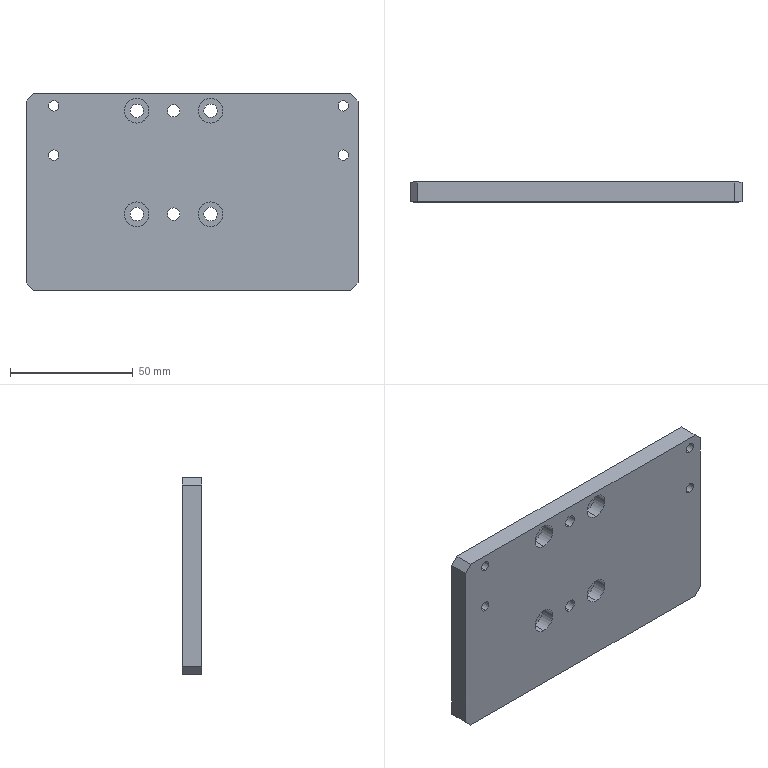Part | SolidWorks | features HoleWzd 3, Chamfer 1, Extrusion 1 | 1 solid | 42 faces | box 135 x 8 x 80 mm | volume 83489 mm3 | cylinder 28 | plane 14 | commonest cylinder face diameters 4.2 x8 5.5 x8 10 x8 5 x4
STEP:
#1=CARTESIAN_POINT('',(60.05,8.,-4.5));
#2=VERTEX_POINT('',#1);
#3=CARTESIAN_POINT('',(60.05,8.,-9.5));
#4=VERTEX_POINT('',#3);
#5=CARTESIAN_POINT('',(60.05,8.,-7.));
#6=DIRECTION('',(0.,-1.,0.));
#7=DIRECTION('',(0.,0.,-1.));
#8=AXIS2_PLACEMENT_3D('',#5,#6,#7);
#9=CIRCLE('',#8,2.5);
#10=EDGE_CURVE('',#2,#4,#9,.T.);
#11=ORIENTED_EDGE('',*,*,#10,.F.);
#12=CARTESIAN_POINT('',(60.05,0.,-4.5));
#13=VERTEX_POINT('',#12);
#14=CARTESIAN_POINT('',(60.05,0.,-4.5));
#15=DIRECTION('',(0.,-1.,0.));
#16=VECTOR('',#15,1000.);
#17=LINE('',#14,#16);
#18=EDGE_CURVE('',#2,#13,#17,.T.);
#19=ORIENTED_EDGE('',*,*,#18,.T.);
#20=CARTESIAN_POINT('',(60.05,0.,-9.5));
#21=VERTEX_POINT('',#20);
#22=CARTESIAN_POINT('',(60.05,0.,-7.));
#23=DIRECTION('',(0.,-1.,0.));
#24=DIRECTION('',(0.,0.,-1.));
#25=AXIS2_PLACEMENT_3D('',#22,#23,#24);
#26=CIRCLE('',#25,2.5);
#27=EDGE_CURVE('',#13,#21,#26,.T.);
#28=ORIENTED_EDGE('',*,*,#27,.T.);
#29=CARTESIAN_POINT('',(60.05,0.,-9.5));
#30=DIRECTION('',(0.,-1.,0.));
#31=VECTOR('',#30,1000.);
#32=LINE('',#29,#31);
#33=EDGE_CURVE('',#4,#21,#32,.T.);
#34=ORIENTED_EDGE('',*,*,#33,.F.);
#35=EDGE_LOOP('',(#11,#19,#28,#34));
#36=FACE_OUTER_BOUND('',#35,.T.);
#37=CARTESIAN_POINT('',(60.05,0.,-7.));
#38=DIRECTION('',(0.,-1.,0.));
#39=DIRECTION('',(0.,0.,-1.));
#40=AXIS2_PLACEMENT_3D('',#37,#38,#39);
#41=CYLINDRICAL_SURFACE('',#40,2.5);
#42=ADVANCED_FACE('',(#36),#41,.F.);
#43=CARTESIAN_POINT('',(60.05,8.,-46.5));
#44=VERTEX_POINT('',#43);
#45=CARTESIAN_POINT('',(60.05,8.,-51.5));
#46=VERTEX_POINT('',#45);
#47=CARTESIAN_POINT('',(60.05,8.,-49.));
#48=DIRECTION('',(0.,-1.,0.));
#49=DIRECTION('',(0.,0.,-1.));
#50=AXIS2_PLACEMENT_3D('',#47,#48,#49);
#51=CIRCLE('',#50,2.5);
#52=EDGE_CURVE('',#44,#46,#51,.T.);
#53=ORIENTED_EDGE('',*,*,#52,.F.);
#54=CARTESIAN_POINT('',(60.05,0.,-46.5));
#55=VERTEX_POINT('',#54);
#56=CARTESIAN_POINT('',(60.05,0.,-46.5));
#57=DIRECTION('',(0.,-1.,0.));
#58=VECTOR('',#57,1000.);
#59=LINE('',#56,#58);
#60=EDGE_CURVE('',#44,#55,#59,.T.);
#61=ORIENTED_EDGE('',*,*,#60,.T.);
#62=CARTESIAN_POINT('',(60.05,0.,-51.5));
#63=VERTEX_POINT('',#62);
#64=CARTESIAN_POINT('',(60.05,0.,-49.));
#65=DIRECTION('',(0.,-1.,0.));
#66=DIRECTION('',(0.,0.,-1.));
#67=AXIS2_PLACEMENT_3D('',#64,#65,#66);
#68=CIRCLE('',#67,2.5);
#69=EDGE_CURVE('',#55,#63,#68,.T.);
#70=ORIENTED_EDGE('',*,*,#69,.T.);
#71=CARTESIAN_POINT('',(60.05,0.,-51.5));
#72=DIRECTION('',(0.,-1.,0.));
#73=VECTOR('',#72,1000.);
#74=LINE('',#71,#73);
#75=EDGE_CURVE('',#46,#63,#74,.T.);
#76=ORIENTED_EDGE('',*,*,#75,.F.);
#77=EDGE_LOOP('',(#53,#61,#70,#76));
#78=FACE_OUTER_BOUND('',#77,.T.);
#79=CARTESIAN_POINT('',(60.05,0.,-49.));
#80=DIRECTION('',(0.,-1.,0.));
#81=DIRECTION('',(0.,0.,-1.));
#82=AXIS2_PLACEMENT_3D('',#79,#80,#81);
#83=CYLINDRICAL_SURFACE('',#82,2.5);
#84=ADVANCED_FACE('',(#78),#83,.F.);
#85=CARTESIAN_POINT('',(129.,0.,-27.1));
#86=VERTEX_POINT('',#85);
#87=CARTESIAN_POINT('',(129.,0.,-22.9));
#88=VERTEX_POINT('',#87);
#89=CARTESIAN_POINT('',(129.,0.,-25.));
#90=DIRECTION('',(0.,1.,0.));
#91=DIRECTION('',(0.,0.,1.));
#92=AXIS2_PLACEMENT_3D('',#89,#90,#91);
#93=CIRCLE('',#92,2.1);
#94=EDGE_CURVE('',#86,#88,#93,.T.);
#95=ORIENTED_EDGE('',*,*,#94,.F.);
#96=CARTESIAN_POINT('',(129.,8.,-27.1));
#97=VERTEX_POINT('',#96);
#98=CARTESIAN_POINT('',(129.,8.,-27.1));
#99=DIRECTION('',(0.,1.,0.));
#100=VECTOR('',#99,1000.);
#101=LINE('',#98,#100);
#102=EDGE_CURVE('',#86,#97,#101,.T.);
#103=ORIENTED_EDGE('',*,*,#102,.T.);
#104=CARTESIAN_POINT('',(129.,8.,-22.9));
#105=VERTEX_POINT('',#104);
#106=CARTESIAN_POINT('',(129.,8.,-25.));
#107=DIRECTION('',(0.,1.,0.));
#108=DIRECTION('',(0.,0.,1.));
#109=AXIS2_PLACEMENT_3D('',#106,#107,#108);
#110=CIRCLE('',#109,2.1);
#111=EDGE_CURVE('',#97,#105,#110,.T.);
#112=ORIENTED_EDGE('',*,*,#111,.T.);
#113=CARTESIAN_POINT('',(129.,8.,-22.9));
#114=DIRECTION('',(0.,1.,0.));
#115=VECTOR('',#114,1000.);
#116=LINE('',#113,#115);
#117=EDGE_CURVE('',#88,#105,#116,.T.);
#118=ORIENTED_EDGE('',*,*,#117,.F.);
#119=EDGE_LOOP('',(#95,#103,#112,#118));
#120=FACE_OUTER_BOUND('',#119,.T.);
#121=CARTESIAN_POINT('',(129.,8.,-25.));
#122=DIRECTION('',(0.,1.,0.));
#123=DIRECTION('',(0.,0.,1.));
#124=AXIS2_PLACEMENT_3D('',#121,#122,#123);
#125=CYLINDRICAL_SURFACE('',#124,2.1);
#126=ADVANCED_FACE('',(#120),#125,.F.);
#127=CARTESIAN_POINT('',(129.,0.,-7.1));
#128=VERTEX_POINT('',#127);
#129=CARTESIAN_POINT('',(129.,0.,-2.9));
#130=VERTEX_POINT('',#129);
#131=CARTESIAN_POINT('',(129.,0.,-5.));
#132=DIRECTION('',(0.,1.,0.));
#133=DIRECTION('',(0.,0.,1.));
#134=AXIS2_PLACEMENT_3D('',#131,#132,#133);
#135=CIRCLE('',#134,2.1);
#136=EDGE_CURVE('',#128,#130,#135,.T.);
#137=ORIENTED_EDGE('',*,*,#136,.F.);
#138=CARTESIAN_POINT('',(129.,8.,-7.1));
#139=VERTEX_POINT('',#138);
#140=CARTESIAN_POINT('',(129.,8.,-7.1));
#141=DIRECTION('',(0.,1.,0.));
#142=VECTOR('',#141,1000.);
#143=LINE('',#140,#142);
#144=EDGE_CURVE('',#128,#139,#143,.T.);
#145=ORIENTED_EDGE('',*,*,#144,.T.);
#146=CARTESIAN_POINT('',(129.,8.,-2.9));
#147=VERTEX_POINT('',#146);
#148=CARTESIAN_POINT('',(129.,8.,-5.));
#149=DIRECTION('',(0.,1.,0.));
#150=DIRECTION('',(0.,0.,1.));
#151=AXIS2_PLACEMENT_3D('',#148,#149,#150);
#152=CIRCLE('',#151,2.1);
#153=EDGE_CURVE('',#139,#147,#152,.T.);
#154=ORIENTED_EDGE('',*,*,#153,.T.);
#155=CARTESIAN_POINT('',(129.,8.,-2.9));
#156=DIRECTION('',(0.,1.,0.));
#157=VECTOR('',#156,1000.);
#158=LINE('',#155,#157);
#159=EDGE_CURVE('',#130,#147,#158,.T.);
#160=ORIENTED_EDGE('',*,*,#159,.F.);
#161=EDGE_LOOP('',(#137,#145,#154,#160));
#162=FACE_OUTER_BOUND('',#161,.T.);
#163=CARTESIAN_POINT('',(129.,8.,-5.));
#164=DIRECTION('',(0.,1.,0.));
#165=DIRECTION('',(0.,0.,1.));
#166=AXIS2_PLACEMENT_3D('',#163,#164,#165);
#167=CYLINDRICAL_SURFACE('',#166,2.1);
#168=ADVANCED_FACE('',(#162),#167,.F.);
#169=CARTESIAN_POINT('',(11.3,0.,-27.1));
#170=VERTEX_POINT('',#169);
#171=CARTESIAN_POINT('',(11.3,0.,-22.9));
#172=VERTEX_POINT('',#171);
#173=CARTESIAN_POINT('',(11.3,0.,-25.));
#174=DIRECTION('',(0.,1.,0.));
#175=DIRECTION('',(0.,0.,1.));
#176=AXIS2_PLACEMENT_3D('',#173,#174,#175);
#177=CIRCLE('',#176,2.1);
#178=EDGE_CURVE('',#170,#172,#177,.T.);
#179=ORIENTED_EDGE('',*,*,#178,.F.);
#180=CARTESIAN_POINT('',(11.3,8.,-27.1));
#181=VERTEX_POINT('',#180);
#182=CARTESIAN_POINT('',(11.3,8.,-27.1));
#183=DIRECTION('',(0.,1.,0.));
#184=VECTOR('',#183,1000.);
#185=LINE('',#182,#184);
#186=EDGE_CURVE('',#170,#181,#185,.T.);
#187=ORIENTED_EDGE('',*,*,#186,.T.);
#188=CARTESIAN_POINT('',(11.3,8.,-22.9));
#189=VERTEX_POINT('',#188);
#190=CARTESIAN_POINT('',(11.3,8.,-25.));
#191=DIRECTION('',(0.,1.,0.));
#192=DIRECTION('',(0.,0.,1.));
#193=AXIS2_PLACEMENT_3D('',#190,#191,#192);
#194=CIRCLE('',#193,2.1);
#195=EDGE_CURVE('',#181,#189,#194,.T.);
#196=ORIENTED_EDGE('',*,*,#195,.T.);
#197=CARTESIAN_POINT('',(11.3,8.,-22.9));
#198=DIRECTION('',(0.,1.,0.));
#199=VECTOR('',#198,1000.);
#200=LINE('',#197,#199);
#201=EDGE_CURVE('',#172,#189,#200,.T.);
#202=ORIENTED_EDGE('',*,*,#201,.F.);
#203=EDGE_LOOP('',(#179,#187,#196,#202));
#204=FACE_OUTER_BOUND('',#203,.T.);
#205=CARTESIAN_POINT('',(11.3,8.,-25.));
#206=DIRECTION('',(0.,1.,0.));
#207=DIRECTION('',(0.,0.,1.));
#208=AXIS2_PLACEMENT_3D('',#205,#206,#207);
#209=CYLINDRICAL_SURFACE('',#208,2.1);
#210=ADVANCED_FACE('',(#204),#209,.F.);
#211=CARTESIAN_POINT('',(11.3,0.,-7.1));
#212=VERTEX_POINT('',#211);
#213=CARTESIAN_POINT('',(11.3,0.,-2.9));
#214=VERTEX_POINT('',#213);
#215=CARTESIAN_POINT('',(11.3,0.,-5.));
#216=DIRECTION('',(0.,1.,0.));
#217=DIRECTION('',(0.,0.,1.));
#218=AXIS2_PLACEMENT_3D('',#215,#216,#217);
#219=CIRCLE('',#218,2.1);
#220=EDGE_CURVE('',#212,#214,#219,.T.);
#221=ORIENTED_EDGE('',*,*,#220,.F.);
#222=CARTESIAN_POINT('',(11.3,8.,-7.1));
#223=VERTEX_POINT('',#222);
#224=CARTESIAN_POINT('',(11.3,8.,-7.1));
#225=DIRECTION('',(0.,1.,0.));
#226=VECTOR('',#225,1000.);
#227=LINE('',#224,#226);
#228=EDGE_CURVE('',#212,#223,#227,.T.);
#229=ORIENTED_EDGE('',*,*,#228,.T.);
#230=CARTESIAN_POINT('',(11.3,8.,-2.9));
#231=VERTEX_POINT('',#230);
#232=CARTESIAN_POINT('',(11.3,8.,-5.));
#233=DIRECTION('',(0.,1.,0.));
#234=DIRECTION('',(0.,0.,1.));
#235=AXIS2_PLACEMENT_3D('',#232,#233,#234);
#236=CIRCLE('',#235,2.1);
#237=EDGE_CURVE('',#223,#231,#236,.T.);
#238=ORIENTED_EDGE('',*,*,#237,.T.);
#239=CARTESIAN_POINT('',(11.3,8.,-2.9));
#240=DIRECTION('',(0.,1.,0.));
#241=VECTOR('',#240,1000.);
#242=LINE('',#239,#241);
#243=EDGE_CURVE('',#214,#231,#242,.T.);
#244=ORIENTED_EDGE('',*,*,#243,.F.);
#245=EDGE_LOOP('',(#221,#229,#238,#244));
#246=FACE_OUTER_BOUND('',#245,.T.);
#247=CARTESIAN_POINT('',(11.3,8.,-5.));
#248=DIRECTION('',(0.,1.,0.));
#249=DIRECTION('',(0.,0.,1.));
#250=AXIS2_PLACEMENT_3D('',#247,#248,#249);
#251=CYLINDRICAL_SURFACE('',#250,2.1);
#252=ADVANCED_FACE('',(#246),#251,.F.);
#253=CARTESIAN_POINT('',(75.05,5.7,-44.));
#254=VERTEX_POINT('',#253);
#255=CARTESIAN_POINT('',(75.05,5.7,-54.));
#256=VERTEX_POINT('',#255);
#257=CARTESIAN_POINT('',(75.05,5.7,-49.));
#258=DIRECTION('',(0.,-1.,0.));
#259=DIRECTION('',(0.,0.,-1.));
#260=AXIS2_PLACEMENT_3D('',#257,#258,#259);
#261=CIRCLE('',#260,5.);
#262=EDGE_CURVE('',#254,#256,#261,.T.);
#263=ORIENTED_EDGE('',*,*,#262,.F.);
#264=CARTESIAN_POINT('',(75.05,0.,-44.));
#265=VERTEX_POINT('',#264);
#266=CARTESIAN_POINT('',(75.05,0.,-44.));
#267=DIRECTION('',(0.,-1.,0.));
#268=VECTOR('',#267,1000.);
#269=LINE('',#266,#268);
#270=EDGE_CURVE('',#254,#265,#269,.T.);
#271=ORIENTED_EDGE('',*,*,#270,.T.);
#272=CARTESIAN_POINT('',(75.05,0.,-54.));
#273=VERTEX_POINT('',#272);
#274=CARTESIAN_POINT('',(75.05,0.,-49.));
#275=DIRECTION('',(0.,-1.,0.));
#276=DIRECTION('',(0.,0.,-1.));
#277=AXIS2_PLACEMENT_3D('',#274,#275,#276);
#278=CIRCLE('',#277,5.);
#279=EDGE_CURVE('',#265,#273,#278,.T.);
#280=ORIENTED_EDGE('',*,*,#279,.T.);
#281=CARTESIAN_POINT('',(75.05,0.,-54.));
#282=DIRECTION('',(0.,-1.,0.));
#283=VECTOR('',#282,1000.);
#284=LINE('',#281,#283);
#285=EDGE_CURVE('',#256,#273,#284,.T.);
#286=ORIENTED_EDGE('',*,*,#285,.F.);
#287=EDGE_LOOP('',(#263,#271,#280,#286));
#288=FACE_OUTER_BOUND('',#287,.T.);
#289=CARTESIAN_POINT('',(75.05,0.,-49.));
#290=DIRECTION('',(0.,-1.,0.));
#291=DIRECTION('',(0.,0.,-1.));
#292=AXIS2_PLACEMENT_3D('',#289,#290,#291);
#293=CYLINDRICAL_SURFACE('',#292,5.);
#294=ADVANCED_FACE('',(#288),#293,.F.);
#295=CARTESIAN_POINT('',(75.05,8.,-46.25));
#296=VERTEX_POINT('',#295);
#297=CARTESIAN_POINT('',(75.05,8.,-51.75));
#298=VERTEX_POINT('',#297);
#299=CARTESIAN_POINT('',(75.05,8.,-49.));
#300=DIRECTION('',(0.,-1.,0.));
#301=DIRECTION('',(0.,0.,-1.));
#302=AXIS2_PLACEMENT_3D('',#299,#300,#301);
#303=CIRCLE('',#302,2.75);
#304=EDGE_CURVE('',#296,#298,#303,.T.);
#305=ORIENTED_EDGE('',*,*,#304,.F.);
#306=CARTESIAN_POINT('',(75.05,5.7,-46.25));
#307=VERTEX_POINT('',#306);
#308=CARTESIAN_POINT('',(75.05,0.,-46.25));
#309=DIRECTION('',(0.,-1.,0.));
#310=VECTOR('',#309,1000.);
#311=LINE('',#308,#310);
#312=EDGE_CURVE('',#296,#307,#311,.T.);
#313=ORIENTED_EDGE('',*,*,#312,.T.);
#314=CARTESIAN_POINT('',(75.05,5.7,-51.75));
#315=VERTEX_POINT('',#314);
#316=CARTESIAN_POINT('',(75.05,5.7,-49.));
#317=DIRECTION('',(0.,-1.,0.));
#318=DIRECTION('',(0.,0.,-1.));
#319=AXIS2_PLACEMENT_3D('',#316,#317,#318);
#320=CIRCLE('',#319,2.75);
#321=EDGE_CURVE('',#307,#315,#320,.T.);
#322=ORIENTED_EDGE('',*,*,#321,.T.);
#323=CARTESIAN_POINT('',(75.05,0.,-51.75));
#324=DIRECTION('',(0.,-1.,0.));
#325=VECTOR('',#324,1000.);
#326=LINE('',#323,#325);
#327=EDGE_CURVE('',#298,#315,#326,.T.);
#328=ORIENTED_EDGE('',*,*,#327,.F.);
#329=EDGE_LOOP('',(#305,#313,#322,#328));
#330=FACE_OUTER_BOUND('',#329,.T.);
#331=CARTESIAN_POINT('',(75.05,0.,-49.));
#332=DIRECTION('',(0.,-1.,0.));
#333=DIRECTION('',(0.,0.,-1.));
#334=AXIS2_PLACEMENT_3D('',#331,#332,#333);
#335=CYLINDRICAL_SURFACE('',#334,2.75);
#336=ADVANCED_FACE('',(#330),#335,.F.);
#337=CARTESIAN_POINT('',(45.05,5.7,-44.));
#338=VERTEX_POINT('',#337);
#339=CARTESIAN_POINT('',(45.05,5.7,-54.));
#340=VERTEX_POINT('',#339);
#341=CARTESIAN_POINT('',(45.05,5.7,-49.));
#342=DIRECTION('',(0.,-1.,0.));
#343=DIRECTION('',(0.,0.,-1.));
#344=AXIS2_PLACEMENT_3D('',#341,#342,#343);
#345=CIRCLE('',#344,5.);
#346=EDGE_CURVE('',#338,#340,#345,.T.);
#347=ORIENTED_EDGE('',*,*,#346,.F.);
#348=CARTESIAN_POINT('',(45.05,0.,-44.));
#349=VERTEX_POINT('',#348);
#350=CARTESIAN_POINT('',(45.05,0.,-44.));
#351=DIRECTION('',(0.,-1.,0.));
#352=VECTOR('',#351,1000.);
#353=LINE('',#350,#352);
#354=EDGE_CURVE('',#338,#349,#353,.T.);
#355=ORIENTED_EDGE('',*,*,#354,.T.);
#356=CARTESIAN_POINT('',(45.05,0.,-54.));
#357=VERTEX_POINT('',#356);
#358=CARTESIAN_POINT('',(45.05,0.,-49.));
#359=DIRECTION('',(0.,-1.,0.));
#360=DIRECTION('',(0.,0.,-1.));
#361=AXIS2_PLACEMENT_3D('',#358,#359,#360);
#362=CIRCLE('',#361,5.);
#363=EDGE_CURVE('',#349,#357,#362,.T.);
#364=ORIENTED_EDGE('',*,*,#363,.T.);
#365=CARTESIAN_POINT('',(45.05,0.,-54.));
#366=DIRECTION('',(0.,-1.,0.));
#367=VECTOR('',#366,1000.);
#368=LINE('',#365,#367);
#369=EDGE_CURVE('',#340,#357,#368,.T.);
#370=ORIENTED_EDGE('',*,*,#369,.F.);
#371=EDGE_LOOP('',(#347,#355,#364,#370));
#372=FACE_OUTER_BOUND('',#371,.T.);
#373=CARTESIAN_POINT('',(45.05,0.,-49.));
#374=DIRECTION('',(0.,-1.,0.));
#375=DIRECTION('',(0.,0.,-1.));
#376=AXIS2_PLACEMENT_3D('',#373,#374,#375);
#377=CYLINDRICAL_SURFACE('',#376,5.);
#378=ADVANCED_FACE('',(#372),#377,.F.);
#379=CARTESIAN_POINT('',(45.05,8.,-46.25));
#380=VERTEX_POINT('',#379);
#381=CARTESIAN_POINT('',(45.05,8.,-51.75));
#382=VERTEX_POINT('',#381);
#383=CARTESIAN_POINT('',(45.05,8.,-49.));
#384=DIRECTION('',(0.,-1.,0.));
#385=DIRECTION('',(0.,0.,-1.));
#386=AXIS2_PLACEMENT_3D('',#383,#384,#385);
#387=CIRCLE('',#386,2.75);
#388=EDGE_CURVE('',#380,#382,#387,.T.);
#389=ORIENTED_EDGE('',*,*,#388,.F.);
#390=CARTESIAN_POINT('',(45.05,5.7,-46.25));
#391=VERTEX_POINT('',#390);
#392=CARTESIAN_POINT('',(45.05,0.,-46.25));
#393=DIRECTION('',(0.,-1.,0.));
#394=VECTOR('',#393,1000.);
#395=LINE('',#392,#394);
#396=EDGE_CURVE('',#380,#391,#395,.T.);
#397=ORIENTED_EDGE('',*,*,#396,.T.);
#398=CARTESIAN_POINT('',(45.05,5.7,-51.75));
#399=VERTEX_POINT('',#398);
#400=CARTESIAN_POINT('',(45.05,5.7,-49.));
#401=DIRECTION('',(0.,-1.,0.));
#402=DIRECTION('',(0.,0.,-1.));
#403=AXIS2_PLACEMENT_3D('',#400,#401,#402);
#404=CIRCLE('',#403,2.75);
#405=EDGE_CURVE('',#391,#399,#404,.T.);
#406=ORIENTED_EDGE('',*,*,#405,.T.);
#407=CARTESIAN_POINT('',(45.05,0.,-51.75));
#408=DIRECTION('',(0.,-1.,0.));
#409=VECTOR('',#408,1000.);
#410=LINE('',#407,#409);
#411=EDGE_CURVE('',#382,#399,#410,.T.);
#412=ORIENTED_EDGE('',*,*,#411,.F.);
#413=EDGE_LOOP('',(#389,#397,#406,#412));
#414=FACE_OUTER_BOUND('',#413,.T.);
#415=CARTESIAN_POINT('',(45.05,0.,-49.));
#416=DIRECTION('',(0.,-1.,0.));
#417=DIRECTION('',(0.,0.,-1.));
#418=AXIS2_PLACEMENT_3D('',#415,#416,#417);
#419=CYLINDRICAL_SURFACE('',#418,2.75);
#420=ADVANCED_FACE('',(#414),#419,.F.);
#421=CARTESIAN_POINT('',(45.05,5.7,-2.));
#422=VERTEX_POINT('',#421);
#423=CARTESIAN_POINT('',(45.05,5.7,-12.));
#424=VERTEX_POINT('',#423);
#425=CARTESIAN_POINT('',(45.05,5.7,-7.));
#426=DIRECTION('',(0.,-1.,0.));
#427=DIRECTION('',(0.,0.,-1.));
#428=AXIS2_PLACEMENT_3D('',#425,#426,#427);
#429=CIRCLE('',#428,5.);
#430=EDGE_CURVE('',#422,#424,#429,.T.);
#431=ORIENTED_EDGE('',*,*,#430,.F.);
#432=CARTESIAN_POINT('',(45.05,0.,-2.));
#433=VERTEX_POINT('',#432);
#434=CARTESIAN_POINT('',(45.05,0.,-2.));
#435=DIRECTION('',(0.,-1.,0.));
#436=VECTOR('',#435,1000.);
#437=LINE('',#434,#436);
#438=EDGE_CURVE('',#422,#433,#437,.T.);
#439=ORIENTED_EDGE('',*,*,#438,.T.);
#440=CARTESIAN_POINT('',(45.05,0.,-12.));
#441=VERTEX_POINT('',#440);
#442=CARTESIAN_POINT('',(45.05,0.,-7.));
#443=DIRECTION('',(0.,-1.,0.));
#444=DIRECTION('',(0.,0.,-1.));
#445=AXIS2_PLACEMENT_3D('',#442,#443,#444);
#446=CIRCLE('',#445,5.);
#447=EDGE_CURVE('',#433,#441,#446,.T.);
#448=ORIENTED_EDGE('',*,*,#447,.T.);
#449=CARTESIAN_POINT('',(45.05,0.,-12.));
#450=DIRECTION('',(0.,-1.,0.));
#451=VECTOR('',#450,1000.);
#452=LINE('',#449,#451);
#453=EDGE_CURVE('',#424,#441,#452,.T.);
#454=ORIENTED_EDGE('',*,*,#453,.F.);
#455=EDGE_LOOP('',(#431,#439,#448,#454));
#456=FACE_OUTER_BOUND('',#455,.T.);
#457=CARTESIAN_POINT('',(45.05,0.,-7.));
#458=DIRECTION('',(0.,-1.,0.));
#459=DIRECTION('',(0.,0.,-1.));
#460=AXIS2_PLACEMENT_3D('',#457,#458,#459);
#461=CYLINDRICAL_SURFACE('',#460,5.);
#462=ADVANCED_FACE('',(#456),#461,.F.);
#463=CARTESIAN_POINT('',(45.05,8.,-4.25));
#464=VERTEX_POINT('',#463);
#465=CARTESIAN_POINT('',(45.05,8.,-9.75));
#466=VERTEX_POINT('',#465);
#467=CARTESIAN_POINT('',(45.05,8.,-7.));
#468=DIRECTION('',(0.,-1.,0.));
#469=DIRECTION('',(0.,0.,-1.));
#470=AXIS2_PLACEMENT_3D('',#467,#468,#469);
#471=CIRCLE('',#470,2.75);
#472=EDGE_CURVE('',#464,#466,#471,.T.);
#473=ORIENTED_EDGE('',*,*,#472,.F.);
#474=CARTESIAN_POINT('',(45.05,5.7,-4.25));
#475=VERTEX_POINT('',#474);
#476=CARTESIAN_POINT('',(45.05,0.,-4.25));
#477=DIRECTION('',(0.,-1.,0.));
#478=VECTOR('',#477,1000.);
#479=LINE('',#476,#478);
#480=EDGE_CURVE('',#464,#475,#479,.T.);
#481=ORIENTED_EDGE('',*,*,#480,.T.);
#482=CARTESIAN_POINT('',(45.05,5.7,-9.75));
#483=VERTEX_POINT('',#482);
#484=CARTESIAN_POINT('',(45.05,5.7,-7.));
#485=DIRECTION('',(0.,-1.,0.));
#486=DIRECTION('',(0.,0.,-1.));
#487=AXIS2_PLACEMENT_3D('',#484,#485,#486);
#488=CIRCLE('',#487,2.75);
#489=EDGE_CURVE('',#475,#483,#488,.T.);
#490=ORIENTED_EDGE('',*,*,#489,.T.);
#491=CARTESIAN_POINT('',(45.05,0.,-9.75));
#492=DIRECTION('',(0.,-1.,0.));
#493=VECTOR('',#492,1000.);
#494=LINE('',#491,#493);
#495=EDGE_CURVE('',#466,#483,#494,.T.);
#496=ORIENTED_EDGE('',*,*,#495,.F.);
#497=EDGE_LOOP('',(#473,#481,#490,#496));
#498=FACE_OUTER_BOUND('',#497,.T.);
#499=CARTESIAN_POINT('',(45.05,0.,-7.));
#500=DIRECTION('',(0.,-1.,0.));
#501=DIRECTION('',(0.,0.,-1.));
#502=AXIS2_PLACEMENT_3D('',#499,#500,#501);
#503=CYLINDRICAL_SURFACE('',#502,2.75);
#504=ADVANCED_FACE('',(#498),#503,.F.);
#505=CARTESIAN_POINT('',(75.05,5.7,-2.));
#506=VERTEX_POINT('',#505);
#507=CARTESIAN_POINT('',(75.05,5.7,-12.));
#508=VERTEX_POINT('',#507);
#509=CARTESIAN_POINT('',(75.05,5.7,-7.));
#510=DIRECTION('',(0.,-1.,0.));
#511=DIRECTION('',(0.,0.,-1.));
#512=AXIS2_PLACEMENT_3D('',#509,#510,#511);
#513=CIRCLE('',#512,5.);
#514=EDGE_CURVE('',#506,#508,#513,.T.);
#515=ORIENTED_EDGE('',*,*,#514,.F.);
#516=CARTESIAN_POINT('',(75.05,0.,-2.));
#517=VERTEX_POINT('',#516);
#518=CARTESIAN_POINT('',(75.05,0.,-2.));
#519=DIRECTION('',(0.,-1.,0.));
#520=VECTOR('',#519,1000.);
#521=LINE('',#518,#520);
#522=EDGE_CURVE('',#506,#517,#521,.T.);
#523=ORIENTED_EDGE('',*,*,#522,.T.);
#524=CARTESIAN_POINT('',(75.05,0.,-12.));
#525=VERTEX_POINT('',#524);
#526=CARTESIAN_POINT('',(75.05,0.,-7.));
#527=DIRECTION('',(0.,-1.,0.));
#528=DIRECTION('',(0.,0.,-1.));
#529=AXIS2_PLACEMENT_3D('',#526,#527,#528);
#530=CIRCLE('',#529,5.);
#531=EDGE_CURVE('',#517,#525,#530,.T.);
#532=ORIENTED_EDGE('',*,*,#531,.T.);
#533=CARTESIAN_POINT('',(75.05,0.,-12.));
#534=DIRECTION('',(0.,-1.,0.));
#535=VECTOR('',#534,1000.);
#536=LINE('',#533,#535);
#537=EDGE_CURVE('',#508,#525,#536,.T.);
#538=ORIENTED_EDGE('',*,*,#537,.F.);
#539=EDGE_LOOP('',(#515,#523,#532,#538));
#540=FACE_OUTER_BOUND('',#539,.T.);
#541=CARTESIAN_POINT('',(75.05,0.,-7.));
#542=DIRECTION('',(0.,-1.,0.));
#543=DIRECTION('',(0.,0.,-1.));
#544=AXIS2_PLACEMENT_3D('',#541,#542,#543);
#545=CYLINDRICAL_SURFACE('',#544,5.);
#546=ADVANCED_FACE('',(#540),#545,.F.);
#547=CARTESIAN_POINT('',(75.05,8.,-4.25));
#548=VERTEX_POINT('',#547);
#549=CARTESIAN_POINT('',(75.05,8.,-9.75));
#550=VERTEX_POINT('',#549);
#551=CARTESIAN_POINT('',(75.05,8.,-7.));
#552=DIRECTION('',(0.,-1.,0.));
#553=DIRECTION('',(0.,0.,-1.));
#554=AXIS2_PLACEMENT_3D('',#551,#552,#553);
#555=CIRCLE('',#554,2.75);
#556=EDGE_CURVE('',#548,#550,#555,.T.);
#557=ORIENTED_EDGE('',*,*,#556,.F.);
#558=CARTESIAN_POINT('',(75.05,5.7,-4.25));
#559=VERTEX_POINT('',#558);
#560=CARTESIAN_POINT('',(75.05,0.,-4.25));
#561=DIRECTION('',(0.,-1.,0.));
#562=VECTOR('',#561,1000.);
#563=LINE('',#560,#562);
#564=EDGE_CURVE('',#548,#559,#563,.T.);
#565=ORIENTED_EDGE('',*,*,#564,.T.);
#566=CARTESIAN_POINT('',(75.05,5.7,-9.75));
#567=VERTEX_POINT('',#566);
#568=CARTESIAN_POINT('',(75.05,5.7,-7.));
#569=DIRECTION('',(0.,-1.,0.));
#570=DIRECTION('',(0.,0.,-1.));
#571=AXIS2_PLACEMENT_3D('',#568,#569,#570);
#572=CIRCLE('',#571,2.75);
#573=EDGE_CURVE('',#559,#567,#572,.T.);
#574=ORIENTED_EDGE('',*,*,#573,.T.);
#575=CARTESIAN_POINT('',(75.05,0.,-9.75));
#576=DIRECTION('',(0.,-1.,0.));
#577=VECTOR('',#576,1000.);
#578=LINE('',#575,#577);
#579=EDGE_CURVE('',#550,#567,#578,.T.);
#580=ORIENTED_EDGE('',*,*,#579,.F.);
#581=EDGE_LOOP('',(#557,#565,#574,#580));
#582=FACE_OUTER_BOUND('',#581,.T.);
#583=CARTESIAN_POINT('',(75.05,0.,-7.));
#584=DIRECTION('',(0.,-1.,0.));
#585=DIRECTION('',(0.,0.,-1.));
#586=AXIS2_PLACEMENT_3D('',#583,#584,#585);
#587=CYLINDRICAL_SURFACE('',#586,2.75);
#588=ADVANCED_FACE('',(#582),#587,.F.);
#589=CARTESIAN_POINT('',(0.,0.,-77.));
#590=VERTEX_POINT('',#589);
#591=CARTESIAN_POINT('',(0.,0.,-3.));
#592=VERTEX_POINT('',#591);
#593=CARTESIAN_POINT('',(0.,0.,0.));
#594=DIRECTION('',(0.,0.,1.));
#595=VECTOR('',#594,1000.);
#596=LINE('',#593,#595);
#597=EDGE_CURVE('',#590,#592,#596,.T.);
#598=ORIENTED_EDGE('',*,*,#597,.T.);
#599=CARTESIAN_POINT('',(0.,8.,-3.));
#600=VERTEX_POINT('',#599);
#601=CARTESIAN_POINT('',(0.,8.,-3.));
#602=DIRECTION('',(0.,1.,0.));
#603=VECTOR('',#602,1000.);
#604=LINE('',#601,#603);
#605=EDGE_CURVE('',#592,#600,#604,.T.);
#606=ORIENTED_EDGE('',*,*,#605,.T.);
#607=CARTESIAN_POINT('',(0.,8.,-77.));
#608=VERTEX_POINT('',#607);
#609=CARTESIAN_POINT('',(0.,8.,0.));
#610=DIRECTION('',(0.,0.,1.));
#611=VECTOR('',#610,1000.);
#612=LINE('',#609,#611);
#613=EDGE_CURVE('',#608,#600,#612,.T.);
#614=ORIENTED_EDGE('',*,*,#613,.F.);
#615=CARTESIAN_POINT('',(0.,8.,-77.));
#616=DIRECTION('',(0.,-1.,0.));
#617=VECTOR('',#616,1000.);
#618=LINE('',#615,#617);
#619=EDGE_CURVE('',#608,#590,#618,.T.);
#620=ORIENTED_EDGE('',*,*,#619,.T.);
#621=EDGE_LOOP('',(#598,#606,#614,#620));
#622=FACE_OUTER_BOUND('',#621,.T.);
#623=CARTESIAN_POINT('',(0.,8.,0.));
#624=DIRECTION('',(1.,0.,0.));
#625=DIRECTION('',(0.,0.,-1.));
#626=AXIS2_PLACEMENT_3D('',#623,#624,#625);
#627=PLANE('',#626);
#628=ADVANCED_FACE('',(#622),#627,.F.);
#629=CARTESIAN_POINT('',(3.,8.,0.));
#630=VERTEX_POINT('',#629);
#631=CARTESIAN_POINT('',(132.,8.,0.));
#632=VERTEX_POINT('',#631);
#633=CARTESIAN_POINT('',(0.,8.,0.));
#634=DIRECTION('',(1.,0.,0.));
#635=VECTOR('',#634,1000.);
#636=LINE('',#633,#635);
#637=EDGE_CURVE('',#630,#632,#636,.T.);
#638=ORIENTED_EDGE('',*,*,#637,.F.);
#639=CARTESIAN_POINT('',(3.,0.,0.));
#640=VERTEX_POINT('',#639);
#641=CARTESIAN_POINT('',(3.,8.,0.));
#642=DIRECTION('',(0.,-1.,0.));
#643=VECTOR('',#642,1000.);
#644=LINE('',#641,#643);
#645=EDGE_CURVE('',#630,#640,#644,.T.);
#646=ORIENTED_EDGE('',*,*,#645,.T.);
#647=CARTESIAN_POINT('',(132.,0.,0.));
#648=VERTEX_POINT('',#647);
#649=CARTESIAN_POINT('',(0.,0.,0.));
#650=DIRECTION('',(1.,0.,0.));
#651=VECTOR('',#650,1000.);
#652=LINE('',#649,#651);
#653=EDGE_CURVE('',#640,#648,#652,.T.);
#654=ORIENTED_EDGE('',*,*,#653,.T.);
#655=CARTESIAN_POINT('',(132.,8.,0.));
#656=DIRECTION('',(0.,1.,0.));
#657=VECTOR('',#656,1000.);
#658=LINE('',#655,#657);
#659=EDGE_CURVE('',#648,#632,#658,.T.);
#660=ORIENTED_EDGE('',*,*,#659,.T.);
#661=EDGE_LOOP('',(#638,#646,#654,#660));
#662=FACE_OUTER_BOUND('',#661,.T.);
#663=CARTESIAN_POINT('',(0.,8.,0.));
#664=DIRECTION('',(0.,0.,-1.));
#665=DIRECTION('',(-1.,0.,0.));
#666=AXIS2_PLACEMENT_3D('',#663,#664,#665);
#667=PLANE('',#666);
#668=ADVANCED_FACE('',(#662),#667,.F.);
#669=CARTESIAN_POINT('',(135.,0.,-3.));
#670=VERTEX_POINT('',#669);
#671=CARTESIAN_POINT('',(135.,0.,-77.));
#672=VERTEX_POINT('',#671);
#673=CARTESIAN_POINT('',(135.,0.,0.));
#674=DIRECTION('',(0.,0.,-1.));
#675=VECTOR('',#674,1000.);
#676=LINE('',#673,#675);
#677=EDGE_CURVE('',#670,#672,#676,.T.);
#678=ORIENTED_EDGE('',*,*,#677,.T.);
#679=CARTESIAN_POINT('',(135.,8.,-77.));
#680=VERTEX_POINT('',#679);
#681=CARTESIAN_POINT('',(135.,8.,-77.));
#682=DIRECTION('',(0.,1.,0.));
#683=VECTOR('',#682,1000.);
#684=LINE('',#681,#683);
#685=EDGE_CURVE('',#672,#680,#684,.T.);
#686=ORIENTED_EDGE('',*,*,#685,.T.);
#687=CARTESIAN_POINT('',(135.,8.,-3.));
#688=VERTEX_POINT('',#687);
#689=CARTESIAN_POINT('',(135.,8.,0.));
#690=DIRECTION('',(0.,0.,-1.));
#691=VECTOR('',#690,1000.);
#692=LINE('',#689,#691);
#693=EDGE_CURVE('',#688,#680,#692,.T.);
#694=ORIENTED_EDGE('',*,*,#693,.F.);
#695=CARTESIAN_POINT('',(135.,8.,-3.));
#696=DIRECTION('',(0.,-1.,0.));
#697=VECTOR('',#696,1000.);
#698=LINE('',#695,#697);
#699=EDGE_CURVE('',#688,#670,#698,.T.);
#700=ORIENTED_EDGE('',*,*,#699,.T.);
#701=EDGE_LOOP('',(#678,#686,#694,#700));
#702=FACE_OUTER_BOUND('',#701,.T.);
#703=CARTESIAN_POINT('',(135.,8.,0.));
#704=DIRECTION('',(-1.,0.,0.));
#705=DIRECTION('',(0.,0.,1.));
#706=AXIS2_PLACEMENT_3D('',#703,#704,#705);
#707=PLANE('',#706);
#708=ADVANCED_FACE('',(#702),#707,.F.);
#709=CARTESIAN_POINT('',(132.,0.,-80.));
#710=VERTEX_POINT('',#709);
#711=CARTESIAN_POINT('',(3.,0.,-80.));
#712=VERTEX_POINT('',#711);
#713=CARTESIAN_POINT('',(0.,0.,-80.));
#714=DIRECTION('',(-1.,0.,0.));
#715=VECTOR('',#714,1000.);
#716=LINE('',#713,#715);
#717=EDGE_CURVE('',#710,#712,#716,.T.);
#718=ORIENTED_EDGE('',*,*,#717,.T.);
#719=CARTESIAN_POINT('',(3.,8.,-80.));
#720=VERTEX_POINT('',#719);
#721=CARTESIAN_POINT('',(3.,8.,-80.));
#722=DIRECTION('',(0.,1.,0.));
#723=VECTOR('',#722,1000.);
#724=LINE('',#721,#723);
#725=EDGE_CURVE('',#712,#720,#724,.T.);
#726=ORIENTED_EDGE('',*,*,#725,.T.);
#727=CARTESIAN_POINT('',(132.,8.,-80.));
#728=VERTEX_POINT('',#727);
#729=CARTESIAN_POINT('',(0.,8.,-80.));
#730=DIRECTION('',(-1.,0.,0.));
#731=VECTOR('',#730,1000.);
#732=LINE('',#729,#731);
#733=EDGE_CURVE('',#728,#720,#732,.T.);
#734=ORIENTED_EDGE('',*,*,#733,.F.);
#735=CARTESIAN_POINT('',(132.,8.,-80.));
#736=DIRECTION('',(0.,-1.,0.));
#737=VECTOR('',#736,1000.);
#738=LINE('',#735,#737);
#739=EDGE_CURVE('',#728,#710,#738,.T.);
#740=ORIENTED_EDGE('',*,*,#739,.T.);
#741=EDGE_LOOP('',(#718,#726,#734,#740));
#742=FACE_OUTER_BOUND('',#741,.T.);
#743=CARTESIAN_POINT('',(0.,8.,-80.));
#744=DIRECTION('',(0.,0.,1.));
#745=DIRECTION('',(1.,0.,0.));
#746=AXIS2_PLACEMENT_3D('',#743,#744,#745);
#747=PLANE('',#746);
#748=ADVANCED_FACE('',(#742),#747,.F.);
#749=CARTESIAN_POINT('',(60.05,8.,-7.));
#750=DIRECTION('',(0.,-1.,0.));
#751=DIRECTION('',(0.,0.,-1.));
#752=AXIS2_PLACEMENT_3D('',#749,#750,#751);
#753=CIRCLE('',#752,2.5);
#754=EDGE_CURVE('',#4,#2,#753,.T.);
#755=ORIENTED_EDGE('',*,*,#754,.T.);
#756=ORIENTED_EDGE('',*,*,#10,.T.);
#757=EDGE_LOOP('',(#755,#756));
#758=FACE_BOUND('',#757,.T.);
#759=CARTESIAN_POINT('',(60.05,8.,-49.));
#760=DIRECTION('',(0.,-1.,0.));
#761=DIRECTION('',(0.,0.,-1.));
#762=AXIS2_PLACEMENT_3D('',#759,#760,#761);
#763=CIRCLE('',#762,2.5);
#764=EDGE_CURVE('',#46,#44,#763,.T.);
#765=ORIENTED_EDGE('',*,*,#764,.T.);
#766=ORIENTED_EDGE('',*,*,#52,.T.);
#767=EDGE_LOOP('',(#765,#766));
#768=FACE_BOUND('',#767,.T.);
#769=CARTESIAN_POINT('',(129.,8.,-25.));
#770=DIRECTION('',(0.,1.,0.));
#771=DIRECTION('',(0.,0.,1.));
#772=AXIS2_PLACEMENT_3D('',#769,#770,#771);
#773=CIRCLE('',#772,2.1);
#774=EDGE_CURVE('',#105,#97,#773,.T.);
#775=ORIENTED_EDGE('',*,*,#774,.F.);
#776=ORIENTED_EDGE('',*,*,#111,.F.);
#777=EDGE_LOOP('',(#775,#776));
#778=FACE_BOUND('',#777,.T.);
#779=CARTESIAN_POINT('',(129.,8.,-5.));
#780=DIRECTION('',(0.,1.,0.));
#781=DIRECTION('',(0.,0.,1.));
#782=AXIS2_PLACEMENT_3D('',#779,#780,#781);
#783=CIRCLE('',#782,2.1);
#784=EDGE_CURVE('',#147,#139,#783,.T.);
#785=ORIENTED_EDGE('',*,*,#784,.F.);
#786=ORIENTED_EDGE('',*,*,#153,.F.);
#787=EDGE_LOOP('',(#785,#786));
#788=FACE_BOUND('',#787,.T.);
#789=CARTESIAN_POINT('',(11.3,8.,-25.));
#790=DIRECTION('',(0.,1.,0.));
#791=DIRECTION('',(0.,0.,1.));
#792=AXIS2_PLACEMENT_3D('',#789,#790,#791);
#793=CIRCLE('',#792,2.1);
#794=EDGE_CURVE('',#189,#181,#793,.T.);
#795=ORIENTED_EDGE('',*,*,#794,.F.);
#796=ORIENTED_EDGE('',*,*,#195,.F.);
#797=EDGE_LOOP('',(#795,#796));
#798=FACE_BOUND('',#797,.T.);
#799=CARTESIAN_POINT('',(11.3,8.,-5.));
#800=DIRECTION('',(0.,1.,0.));
#801=DIRECTION('',(0.,0.,1.));
#802=AXIS2_PLACEMENT_3D('',#799,#800,#801);
#803=CIRCLE('',#802,2.1);
#804=EDGE_CURVE('',#231,#223,#803,.T.);
#805=ORIENTED_EDGE('',*,*,#804,.F.);
#806=ORIENTED_EDGE('',*,*,#237,.F.);
#807=EDGE_LOOP('',(#805,#806));
#808=FACE_BOUND('',#807,.T.);
#809=CARTESIAN_POINT('',(75.05,8.,-49.));
#810=DIRECTION('',(0.,-1.,0.));
#811=DIRECTION('',(0.,0.,-1.));
#812=AXIS2_PLACEMENT_3D('',#809,#810,#811);
#813=CIRCLE('',#812,2.75);
#814=EDGE_CURVE('',#298,#296,#813,.T.);
#815=ORIENTED_EDGE('',*,*,#814,.T.);
#816=ORIENTED_EDGE('',*,*,#304,.T.);
#817=EDGE_LOOP('',(#815,#816));
#818=FACE_BOUND('',#817,.T.);
#819=CARTESIAN_POINT('',(45.05,8.,-49.));
#820=DIRECTION('',(0.,-1.,0.));
#821=DIRECTION('',(0.,0.,-1.));
#822=AXIS2_PLACEMENT_3D('',#819,#820,#821);
#823=CIRCLE('',#822,2.75);
#824=EDGE_CURVE('',#382,#380,#823,.T.);
#825=ORIENTED_EDGE('',*,*,#824,.T.);
#826=ORIENTED_EDGE('',*,*,#388,.T.);
#827=EDGE_LOOP('',(#825,#826));
#828=FACE_BOUND('',#827,.T.);
#829=CARTESIAN_POINT('',(45.05,8.,-7.));
#830=DIRECTION('',(0.,-1.,0.));
#831=DIRECTION('',(0.,0.,-1.));
#832=AXIS2_PLACEMENT_3D('',#829,#830,#831);
#833=CIRCLE('',#832,2.75);
#834=EDGE_CURVE('',#466,#464,#833,.T.);
#835=ORIENTED_EDGE('',*,*,#834,.T.);
#836=ORIENTED_EDGE('',*,*,#472,.T.);
#837=EDGE_LOOP('',(#835,#836));
#838=FACE_BOUND('',#837,.T.);
#839=CARTESIAN_POINT('',(75.05,8.,-7.));
#840=DIRECTION('',(0.,-1.,0.));
#841=DIRECTION('',(0.,0.,-1.));
#842=AXIS2_PLACEMENT_3D('',#839,#840,#841);
#843=CIRCLE('',#842,2.75);
#844=EDGE_CURVE('',#550,#548,#843,.T.);
#845=ORIENTED_EDGE('',*,*,#844,.T.);
#846=ORIENTED_EDGE('',*,*,#556,.T.);
#847=EDGE_LOOP('',(#845,#846));
#848=FACE_BOUND('',#847,.T.);
#849=ORIENTED_EDGE('',*,*,#613,.T.);
#850=CARTESIAN_POINT('',(3.,8.,0.));
#851=DIRECTION('',(0.7071,0.,0.7071));
#852=VECTOR('',#851,1000.);
#853=LINE('',#850,#852);
#854=EDGE_CURVE('',#600,#630,#853,.T.);
#855=ORIENTED_EDGE('',*,*,#854,.T.);
#856=ORIENTED_EDGE('',*,*,#637,.T.);
#857=CARTESIAN_POINT('',(135.,8.,-3.));
#858=DIRECTION('',(0.7071,0.,-0.7071));
#859=VECTOR('',#858,1000.);
#860=LINE('',#857,#859);
#861=EDGE_CURVE('',#632,#688,#860,.T.);
#862=ORIENTED_EDGE('',*,*,#861,.T.);
#863=ORIENTED_EDGE('',*,*,#693,.T.);
#864=CARTESIAN_POINT('',(132.,8.,-80.));
#865=DIRECTION('',(-0.7071,0.,-0.7071));
#866=VECTOR('',#865,1000.);
#867=LINE('',#864,#866);
#868=EDGE_CURVE('',#680,#728,#867,.T.);
#869=ORIENTED_EDGE('',*,*,#868,.T.);
#870=ORIENTED_EDGE('',*,*,#733,.T.);
#871=CARTESIAN_POINT('',(0.,8.,-77.));
#872=DIRECTION('',(-0.7071,0.,0.7071));
#873=VECTOR('',#872,1000.);
#874=LINE('',#871,#873);
#875=EDGE_CURVE('',#720,#608,#874,.T.);
#876=ORIENTED_EDGE('',*,*,#875,.T.);
#877=EDGE_LOOP('',(#849,#855,#856,#862,#863,#869,#870,#876));
#878=FACE_OUTER_BOUND('',#877,.T.);
#879=CARTESIAN_POINT('',(0.,8.,0.));
#880=DIRECTION('',(0.,-1.,0.));
#881=DIRECTION('',(0.,0.,-1.));
#882=AXIS2_PLACEMENT_3D('',#879,#880,#881);
#883=PLANE('',#882);
#884=ADVANCED_FACE('',(#758,#768,#778,#788,#798,#808,#818,#828,#838,#848,#878),#883,.F.);
#885=CARTESIAN_POINT('',(60.05,0.,-7.));
#886=DIRECTION('',(0.,-1.,0.));
#887=DIRECTION('',(0.,0.,-1.));
#888=AXIS2_PLACEMENT_3D('',#885,#886,#887);
#889=CIRCLE('',#888,2.5);
#890=EDGE_CURVE('',#21,#13,#889,.T.);
#891=ORIENTED_EDGE('',*,*,#890,.F.);
#892=ORIENTED_EDGE('',*,*,#27,.F.);
#893=EDGE_LOOP('',(#891,#892));
#894=FACE_BOUND('',#893,.T.);
#895=CARTESIAN_POINT('',(60.05,0.,-49.));
#896=DIRECTION('',(0.,-1.,0.));
#897=DIRECTION('',(0.,0.,-1.));
#898=AXIS2_PLACEMENT_3D('',#895,#896,#897);
#899=CIRCLE('',#898,2.5);
#900=EDGE_CURVE('',#63,#55,#899,.T.);
#901=ORIENTED_EDGE('',*,*,#900,.F.);
#902=ORIENTED_EDGE('',*,*,#69,.F.);
#903=EDGE_LOOP('',(#901,#902));
#904=FACE_BOUND('',#903,.T.);
#905=CARTESIAN_POINT('',(129.,0.,-25.));
#906=DIRECTION('',(0.,1.,0.));
#907=DIRECTION('',(0.,0.,1.));
#908=AXIS2_PLACEMENT_3D('',#905,#906,#907);
#909=CIRCLE('',#908,2.1);
#910=EDGE_CURVE('',#88,#86,#909,.T.);
#911=ORIENTED_EDGE('',*,*,#910,.T.);
#912=ORIENTED_EDGE('',*,*,#94,.T.);
#913=EDGE_LOOP('',(#911,#912));
#914=FACE_BOUND('',#913,.T.);
#915=CARTESIAN_POINT('',(129.,0.,-5.));
#916=DIRECTION('',(0.,1.,0.));
#917=DIRECTION('',(0.,0.,1.));
#918=AXIS2_PLACEMENT_3D('',#915,#916,#917);
#919=CIRCLE('',#918,2.1);
#920=EDGE_CURVE('',#130,#128,#919,.T.);
#921=ORIENTED_EDGE('',*,*,#920,.T.);
#922=ORIENTED_EDGE('',*,*,#136,.T.);
#923=EDGE_LOOP('',(#921,#922));
#924=FACE_BOUND('',#923,.T.);
#925=CARTESIAN_POINT('',(11.3,0.,-25.));
#926=DIRECTION('',(0.,1.,0.));
#927=DIRECTION('',(0.,0.,1.));
#928=AXIS2_PLACEMENT_3D('',#925,#926,#927);
#929=CIRCLE('',#928,2.1);
#930=EDGE_CURVE('',#172,#170,#929,.T.);
#931=ORIENTED_EDGE('',*,*,#930,.T.);
#932=ORIENTED_EDGE('',*,*,#178,.T.);
#933=EDGE_LOOP('',(#931,#932));
#934=FACE_BOUND('',#933,.T.);
#935=CARTESIAN_POINT('',(11.3,0.,-5.));
#936=DIRECTION('',(0.,1.,0.));
#937=DIRECTION('',(0.,0.,1.));
#938=AXIS2_PLACEMENT_3D('',#935,#936,#937);
#939=CIRCLE('',#938,2.1);
#940=EDGE_CURVE('',#214,#212,#939,.T.);
#941=ORIENTED_EDGE('',*,*,#940,.T.);
#942=ORIENTED_EDGE('',*,*,#220,.T.);
#943=EDGE_LOOP('',(#941,#942));
#944=FACE_BOUND('',#943,.T.);
#945=CARTESIAN_POINT('',(75.05,0.,-49.));
#946=DIRECTION('',(0.,-1.,0.));
#947=DIRECTION('',(0.,0.,-1.));
#948=AXIS2_PLACEMENT_3D('',#945,#946,#947);
#949=CIRCLE('',#948,5.);
#950=EDGE_CURVE('',#273,#265,#949,.T.);
#951=ORIENTED_EDGE('',*,*,#950,.F.);
#952=ORIENTED_EDGE('',*,*,#279,.F.);
#953=EDGE_LOOP('',(#951,#952));
#954=FACE_BOUND('',#953,.T.);
#955=CARTESIAN_POINT('',(45.05,0.,-49.));
#956=DIRECTION('',(0.,-1.,0.));
#957=DIRECTION('',(0.,0.,-1.));
#958=AXIS2_PLACEMENT_3D('',#955,#956,#957);
#959=CIRCLE('',#958,5.);
#960=EDGE_CURVE('',#357,#349,#959,.T.);
#961=ORIENTED_EDGE('',*,*,#960,.F.);
#962=ORIENTED_EDGE('',*,*,#363,.F.);
#963=EDGE_LOOP('',(#961,#962));
#964=FACE_BOUND('',#963,.T.);
#965=CARTESIAN_POINT('',(45.05,0.,-7.));
#966=DIRECTION('',(0.,-1.,0.));
#967=DIRECTION('',(0.,0.,-1.));
#968=AXIS2_PLACEMENT_3D('',#965,#966,#967);
#969=CIRCLE('',#968,5.);
#970=EDGE_CURVE('',#441,#433,#969,.T.);
#971=ORIENTED_EDGE('',*,*,#970,.F.);
#972=ORIENTED_EDGE('',*,*,#447,.F.);
#973=EDGE_LOOP('',(#971,#972));
#974=FACE_BOUND('',#973,.T.);
#975=CARTESIAN_POINT('',(75.05,0.,-7.));
#976=DIRECTION('',(0.,-1.,0.));
#977=DIRECTION('',(0.,0.,-1.));
#978=AXIS2_PLACEMENT_3D('',#975,#976,#977);
#979=CIRCLE('',#978,5.);
#980=EDGE_CURVE('',#525,#517,#979,.T.);
#981=ORIENTED_EDGE('',*,*,#980,.F.);
#982=ORIENTED_EDGE('',*,*,#531,.F.);
#983=EDGE_LOOP('',(#981,#982));
#984=FACE_BOUND('',#983,.T.);
#985=ORIENTED_EDGE('',*,*,#653,.F.);
#986=CARTESIAN_POINT('',(1.5,0.,-1.5));
#987=DIRECTION('',(-0.7071,0.,-0.7071));
#988=VECTOR('',#987,1000.);
#989=LINE('',#986,#988);
#990=EDGE_CURVE('',#640,#592,#989,.T.);
#991=ORIENTED_EDGE('',*,*,#990,.T.);
#992=ORIENTED_EDGE('',*,*,#597,.F.);
#993=CARTESIAN_POINT('',(-38.5,0.,-38.5));
#994=DIRECTION('',(0.7071,0.,-0.7071));
#995=VECTOR('',#994,1000.);
#996=LINE('',#993,#995);
#997=EDGE_CURVE('',#590,#712,#996,.T.);
#998=ORIENTED_EDGE('',*,*,#997,.T.);
#999=ORIENTED_EDGE('',*,*,#717,.F.);
#1000=CARTESIAN_POINT('',(106.,0.,-106.));
#1001=DIRECTION('',(0.7071,0.,0.7071));
#1002=VECTOR('',#1001,1000.);
#1003=LINE('',#1000,#1002);
#1004=EDGE_CURVE('',#710,#672,#1003,.T.);
#1005=ORIENTED_EDGE('',*,*,#1004,.T.);
#1006=ORIENTED_EDGE('',*,*,#677,.F.);
#1007=CARTESIAN_POINT('',(66.,0.,66.));
#1008=DIRECTION('',(-0.7071,0.,0.7071));
#1009=VECTOR('',#1008,1000.);
#1010=LINE('',#1007,#1009);
#1011=EDGE_CURVE('',#670,#648,#1010,.T.);
#1012=ORIENTED_EDGE('',*,*,#1011,.T.);
#1013=EDGE_LOOP('',(#985,#991,#992,#998,#999,#1005,#1006,#1012));
#1014=FACE_OUTER_BOUND('',#1013,.T.);
#1015=CARTESIAN_POINT('',(0.,0.,0.));
#1016=DIRECTION('',(0.,-1.,0.));
#1017=DIRECTION('',(0.,0.,-1.));
#1018=AXIS2_PLACEMENT_3D('',#1015,#1016,#1017);
#1019=PLANE('',#1018);
#1020=ADVANCED_FACE('',(#894,#904,#914,#924,#934,#944,#954,#964,#974,#984,#1014),#1019,.T.);
#1021=ORIENTED_EDGE('',*,*,#564,.F.);
#1022=ORIENTED_EDGE('',*,*,#844,.F.);
#1023=ORIENTED_EDGE('',*,*,#579,.T.);
#1024=CARTESIAN_POINT('',(75.05,5.7,-7.));
#1025=DIRECTION('',(0.,-1.,0.));
#1026=DIRECTION('',(0.,0.,-1.));
#1027=AXIS2_PLACEMENT_3D('',#1024,#1025,#1026);
#1028=CIRCLE('',#1027,2.75);
#1029=EDGE_CURVE('',#567,#559,#1028,.T.);
#1030=ORIENTED_EDGE('',*,*,#1029,.T.);
#1031=EDGE_LOOP('',(#1021,#1022,#1023,#1030));
#1032=FACE_OUTER_BOUND('',#1031,.T.);
#1033=CARTESIAN_POINT('',(75.05,0.,-7.));
#1034=DIRECTION('',(0.,-1.,0.));
#1035=DIRECTION('',(0.,0.,-1.));
#1036=AXIS2_PLACEMENT_3D('',#1033,#1034,#1035);
#1037=CYLINDRICAL_SURFACE('',#1036,2.75);
#1038=ADVANCED_FACE('',(#1032),#1037,.F.);
#1039=ORIENTED_EDGE('',*,*,#1029,.F.);
#1040=ORIENTED_EDGE('',*,*,#573,.F.);
#1041=EDGE_LOOP('',(#1039,#1040));
#1042=FACE_BOUND('',#1041,.T.);
#1043=CARTESIAN_POINT('',(75.05,5.7,-7.));
#1044=DIRECTION('',(0.,-1.,0.));
#1045=DIRECTION('',(0.,0.,-1.));
#1046=AXIS2_PLACEMENT_3D('',#1043,#1044,#1045);
#1047=CIRCLE('',#1046,5.);
#1048=EDGE_CURVE('',#508,#506,#1047,.T.);
#1049=ORIENTED_EDGE('',*,*,#1048,.T.);
#1050=ORIENTED_EDGE('',*,*,#514,.T.);
#1051=EDGE_LOOP('',(#1049,#1050));
#1052=FACE_OUTER_BOUND('',#1051,.T.);
#1053=CARTESIAN_POINT('',(77.8,5.7,-7.));
#1054=DIRECTION('',(0.,1.,0.));
#1055=DIRECTION('',(0.,0.,1.));
#1056=AXIS2_PLACEMENT_3D('',#1053,#1054,#1055);
#1057=PLANE('',#1056);
#1058=ADVANCED_FACE('',(#1042,#1052),#1057,.F.);
#1059=ORIENTED_EDGE('',*,*,#522,.F.);
#1060=ORIENTED_EDGE('',*,*,#1048,.F.);
#1061=ORIENTED_EDGE('',*,*,#537,.T.);
#1062=ORIENTED_EDGE('',*,*,#980,.T.);
#1063=EDGE_LOOP('',(#1059,#1060,#1061,#1062));
#1064=FACE_OUTER_BOUND('',#1063,.T.);
#1065=CARTESIAN_POINT('',(75.05,0.,-7.));
#1066=DIRECTION('',(0.,-1.,0.));
#1067=DIRECTION('',(0.,0.,-1.));
#1068=AXIS2_PLACEMENT_3D('',#1065,#1066,#1067);
#1069=CYLINDRICAL_SURFACE('',#1068,5.);
#1070=ADVANCED_FACE('',(#1064),#1069,.F.);
#1071=ORIENTED_EDGE('',*,*,#480,.F.);
#1072=ORIENTED_EDGE('',*,*,#834,.F.);
#1073=ORIENTED_EDGE('',*,*,#495,.T.);
#1074=CARTESIAN_POINT('',(45.05,5.7,-7.));
#1075=DIRECTION('',(0.,-1.,0.));
#1076=DIRECTION('',(0.,0.,-1.));
#1077=AXIS2_PLACEMENT_3D('',#1074,#1075,#1076);
#1078=CIRCLE('',#1077,2.75);
#1079=EDGE_CURVE('',#483,#475,#1078,.T.);
#1080=ORIENTED_EDGE('',*,*,#1079,.T.);
#1081=EDGE_LOOP('',(#1071,#1072,#1073,#1080));
#1082=FACE_OUTER_BOUND('',#1081,.T.);
#1083=CARTESIAN_POINT('',(45.05,0.,-7.));
#1084=DIRECTION('',(0.,-1.,0.));
#1085=DIRECTION('',(0.,0.,-1.));
#1086=AXIS2_PLACEMENT_3D('',#1083,#1084,#1085);
#1087=CYLINDRICAL_SURFACE('',#1086,2.75);
#1088=ADVANCED_FACE('',(#1082),#1087,.F.);
#1089=ORIENTED_EDGE('',*,*,#1079,.F.);
#1090=ORIENTED_EDGE('',*,*,#489,.F.);
#1091=EDGE_LOOP('',(#1089,#1090));
#1092=FACE_BOUND('',#1091,.T.);
#1093=CARTESIAN_POINT('',(45.05,5.7,-7.));
#1094=DIRECTION('',(0.,-1.,0.));
#1095=DIRECTION('',(0.,0.,-1.));
#1096=AXIS2_PLACEMENT_3D('',#1093,#1094,#1095);
#1097=CIRCLE('',#1096,5.);
#1098=EDGE_CURVE('',#424,#422,#1097,.T.);
#1099=ORIENTED_EDGE('',*,*,#1098,.T.);
#1100=ORIENTED_EDGE('',*,*,#430,.T.);
#1101=EDGE_LOOP('',(#1099,#1100));
#1102=FACE_OUTER_BOUND('',#1101,.T.);
#1103=CARTESIAN_POINT('',(47.8,5.7,-7.));
#1104=DIRECTION('',(0.,1.,0.));
#1105=DIRECTION('',(0.,0.,1.));
#1106=AXIS2_PLACEMENT_3D('',#1103,#1104,#1105);
#1107=PLANE('',#1106);
#1108=ADVANCED_FACE('',(#1092,#1102),#1107,.F.);
#1109=ORIENTED_EDGE('',*,*,#438,.F.);
#1110=ORIENTED_EDGE('',*,*,#1098,.F.);
#1111=ORIENTED_EDGE('',*,*,#453,.T.);
#1112=ORIENTED_EDGE('',*,*,#970,.T.);
#1113=EDGE_LOOP('',(#1109,#1110,#1111,#1112));
#1114=FACE_OUTER_BOUND('',#1113,.T.);
#1115=CARTESIAN_POINT('',(45.05,0.,-7.));
#1116=DIRECTION('',(0.,-1.,0.));
#1117=DIRECTION('',(0.,0.,-1.));
#1118=AXIS2_PLACEMENT_3D('',#1115,#1116,#1117);
#1119=CYLINDRICAL_SURFACE('',#1118,5.);
#1120=ADVANCED_FACE('',(#1114),#1119,.F.);
#1121=ORIENTED_EDGE('',*,*,#396,.F.);
#1122=ORIENTED_EDGE('',*,*,#824,.F.);
#1123=ORIENTED_EDGE('',*,*,#411,.T.);
#1124=CARTESIAN_POINT('',(45.05,5.7,-49.));
#1125=DIRECTION('',(0.,-1.,0.));
#1126=DIRECTION('',(0.,0.,-1.));
#1127=AXIS2_PLACEMENT_3D('',#1124,#1125,#1126);
#1128=CIRCLE('',#1127,2.75);
#1129=EDGE_CURVE('',#399,#391,#1128,.T.);
#1130=ORIENTED_EDGE('',*,*,#1129,.T.);
#1131=EDGE_LOOP('',(#1121,#1122,#1123,#1130));
#1132=FACE_OUTER_BOUND('',#1131,.T.);
#1133=CARTESIAN_POINT('',(45.05,0.,-49.));
#1134=DIRECTION('',(0.,-1.,0.));
#1135=DIRECTION('',(0.,0.,-1.));
#1136=AXIS2_PLACEMENT_3D('',#1133,#1134,#1135);
#1137=CYLINDRICAL_SURFACE('',#1136,2.75);
#1138=ADVANCED_FACE('',(#1132),#1137,.F.);
#1139=ORIENTED_EDGE('',*,*,#1129,.F.);
#1140=ORIENTED_EDGE('',*,*,#405,.F.);
#1141=EDGE_LOOP('',(#1139,#1140));
#1142=FACE_BOUND('',#1141,.T.);
#1143=CARTESIAN_POINT('',(45.05,5.7,-49.));
#1144=DIRECTION('',(0.,-1.,0.));
#1145=DIRECTION('',(0.,0.,-1.));
#1146=AXIS2_PLACEMENT_3D('',#1143,#1144,#1145);
#1147=CIRCLE('',#1146,5.);
#1148=EDGE_CURVE('',#340,#338,#1147,.T.);
#1149=ORIENTED_EDGE('',*,*,#1148,.T.);
#1150=ORIENTED_EDGE('',*,*,#346,.T.);
#1151=EDGE_LOOP('',(#1149,#1150));
#1152=FACE_OUTER_BOUND('',#1151,.T.);
#1153=CARTESIAN_POINT('',(47.8,5.7,-49.));
#1154=DIRECTION('',(0.,1.,0.));
#1155=DIRECTION('',(0.,0.,1.));
#1156=AXIS2_PLACEMENT_3D('',#1153,#1154,#1155);
#1157=PLANE('',#1156);
#1158=ADVANCED_FACE('',(#1142,#1152),#1157,.F.);
#1159=ORIENTED_EDGE('',*,*,#354,.F.);
#1160=ORIENTED_EDGE('',*,*,#1148,.F.);
#1161=ORIENTED_EDGE('',*,*,#369,.T.);
#1162=ORIENTED_EDGE('',*,*,#960,.T.);
#1163=EDGE_LOOP('',(#1159,#1160,#1161,#1162));
#1164=FACE_OUTER_BOUND('',#1163,.T.);
#1165=CARTESIAN_POINT('',(45.05,0.,-49.));
#1166=DIRECTION('',(0.,-1.,0.));
#1167=DIRECTION('',(0.,0.,-1.));
#1168=AXIS2_PLACEMENT_3D('',#1165,#1166,#1167);
#1169=CYLINDRICAL_SURFACE('',#1168,5.);
#1170=ADVANCED_FACE('',(#1164),#1169,.F.);
#1171=ORIENTED_EDGE('',*,*,#312,.F.);
#1172=ORIENTED_EDGE('',*,*,#814,.F.);
#1173=ORIENTED_EDGE('',*,*,#327,.T.);
#1174=CARTESIAN_POINT('',(75.05,5.7,-49.));
#1175=DIRECTION('',(0.,-1.,0.));
#1176=DIRECTION('',(0.,0.,-1.));
#1177=AXIS2_PLACEMENT_3D('',#1174,#1175,#1176);
#1178=CIRCLE('',#1177,2.75);
#1179=EDGE_CURVE('',#315,#307,#1178,.T.);
#1180=ORIENTED_EDGE('',*,*,#1179,.T.);
#1181=EDGE_LOOP('',(#1171,#1172,#1173,#1180));
#1182=FACE_OUTER_BOUND('',#1181,.T.);
#1183=CARTESIAN_POINT('',(75.05,0.,-49.));
#1184=DIRECTION('',(0.,-1.,0.));
#1185=DIRECTION('',(0.,0.,-1.));
#1186=AXIS2_PLACEMENT_3D('',#1183,#1184,#1185);
#1187=CYLINDRICAL_SURFACE('',#1186,2.75);
#1188=ADVANCED_FACE('',(#1182),#1187,.F.);
#1189=ORIENTED_EDGE('',*,*,#1179,.F.);
#1190=ORIENTED_EDGE('',*,*,#321,.F.);
#1191=EDGE_LOOP('',(#1189,#1190));
#1192=FACE_BOUND('',#1191,.T.);
#1193=CARTESIAN_POINT('',(75.05,5.7,-49.));
#1194=DIRECTION('',(0.,-1.,0.));
#1195=DIRECTION('',(0.,0.,-1.));
#1196=AXIS2_PLACEMENT_3D('',#1193,#1194,#1195);
#1197=CIRCLE('',#1196,5.);
#1198=EDGE_CURVE('',#256,#254,#1197,.T.);
#1199=ORIENTED_EDGE('',*,*,#1198,.T.);
#1200=ORIENTED_EDGE('',*,*,#262,.T.);
#1201=EDGE_LOOP('',(#1199,#1200));
#1202=FACE_OUTER_BOUND('',#1201,.T.);
#1203=CARTESIAN_POINT('',(77.8,5.7,-49.));
#1204=DIRECTION('',(0.,1.,0.));
#1205=DIRECTION('',(0.,0.,1.));
#1206=AXIS2_PLACEMENT_3D('',#1203,#1204,#1205);
#1207=PLANE('',#1206);
#1208=ADVANCED_FACE('',(#1192,#1202),#1207,.F.);
#1209=ORIENTED_EDGE('',*,*,#270,.F.);
#1210=ORIENTED_EDGE('',*,*,#1198,.F.);
#1211=ORIENTED_EDGE('',*,*,#285,.T.);
#1212=ORIENTED_EDGE('',*,*,#950,.T.);
#1213=EDGE_LOOP('',(#1209,#1210,#1211,#1212));
#1214=FACE_OUTER_BOUND('',#1213,.T.);
#1215=CARTESIAN_POINT('',(75.05,0.,-49.));
#1216=DIRECTION('',(0.,-1.,0.));
#1217=DIRECTION('',(0.,0.,-1.));
#1218=AXIS2_PLACEMENT_3D('',#1215,#1216,#1217);
#1219=CYLINDRICAL_SURFACE('',#1218,5.);
#1220=ADVANCED_FACE('',(#1214),#1219,.F.);
#1221=ORIENTED_EDGE('',*,*,#228,.F.);
#1222=ORIENTED_EDGE('',*,*,#940,.F.);
#1223=ORIENTED_EDGE('',*,*,#243,.T.);
#1224=ORIENTED_EDGE('',*,*,#804,.T.);
#1225=EDGE_LOOP('',(#1221,#1222,#1223,#1224));
#1226=FACE_OUTER_BOUND('',#1225,.T.);
#1227=CARTESIAN_POINT('',(11.3,8.,-5.));
#1228=DIRECTION('',(0.,1.,0.));
#1229=DIRECTION('',(0.,0.,1.));
#1230=AXIS2_PLACEMENT_3D('',#1227,#1228,#1229);
#1231=CYLINDRICAL_SURFACE('',#1230,2.1);
#1232=ADVANCED_FACE('',(#1226),#1231,.F.);
#1233=ORIENTED_EDGE('',*,*,#186,.F.);
#1234=ORIENTED_EDGE('',*,*,#930,.F.);
#1235=ORIENTED_EDGE('',*,*,#201,.T.);
#1236=ORIENTED_EDGE('',*,*,#794,.T.);
#1237=EDGE_LOOP('',(#1233,#1234,#1235,#1236));
#1238=FACE_OUTER_BOUND('',#1237,.T.);
#1239=CARTESIAN_POINT('',(11.3,8.,-25.));
#1240=DIRECTION('',(0.,1.,0.));
#1241=DIRECTION('',(0.,0.,1.));
#1242=AXIS2_PLACEMENT_3D('',#1239,#1240,#1241);
#1243=CYLINDRICAL_SURFACE('',#1242,2.1);
#1244=ADVANCED_FACE('',(#1238),#1243,.F.);
#1245=ORIENTED_EDGE('',*,*,#144,.F.);
#1246=ORIENTED_EDGE('',*,*,#920,.F.);
#1247=ORIENTED_EDGE('',*,*,#159,.T.);
#1248=ORIENTED_EDGE('',*,*,#784,.T.);
#1249=EDGE_LOOP('',(#1245,#1246,#1247,#1248));
#1250=FACE_OUTER_BOUND('',#1249,.T.);
#1251=CARTESIAN_POINT('',(129.,8.,-5.));
#1252=DIRECTION('',(0.,1.,0.));
#1253=DIRECTION('',(0.,0.,1.));
#1254=AXIS2_PLACEMENT_3D('',#1251,#1252,#1253);
#1255=CYLINDRICAL_SURFACE('',#1254,2.1);
#1256=ADVANCED_FACE('',(#1250),#1255,.F.);
#1257=ORIENTED_EDGE('',*,*,#102,.F.);
#1258=ORIENTED_EDGE('',*,*,#910,.F.);
#1259=ORIENTED_EDGE('',*,*,#117,.T.);
#1260=ORIENTED_EDGE('',*,*,#774,.T.);
#1261=EDGE_LOOP('',(#1257,#1258,#1259,#1260));
#1262=FACE_OUTER_BOUND('',#1261,.T.);
#1263=CARTESIAN_POINT('',(129.,8.,-25.));
#1264=DIRECTION('',(0.,1.,0.));
#1265=DIRECTION('',(0.,0.,1.));
#1266=AXIS2_PLACEMENT_3D('',#1263,#1264,#1265);
#1267=CYLINDRICAL_SURFACE('',#1266,2.1);
#1268=ADVANCED_FACE('',(#1262),#1267,.F.);
#1269=ORIENTED_EDGE('',*,*,#854,.F.);
#1270=ORIENTED_EDGE('',*,*,#605,.F.);
#1271=ORIENTED_EDGE('',*,*,#990,.F.);
#1272=ORIENTED_EDGE('',*,*,#645,.F.);
#1273=EDGE_LOOP('',(#1269,#1270,#1271,#1272));
#1274=FACE_OUTER_BOUND('',#1273,.T.);
#1275=CARTESIAN_POINT('',(3.,8.,0.));
#1276=DIRECTION('',(0.7071,0.,-0.7071));
#1277=DIRECTION('',(0.,-1.,0.));
#1278=AXIS2_PLACEMENT_3D('',#1275,#1276,#1277);
#1279=PLANE('',#1278);
#1280=ADVANCED_FACE('',(#1274),#1279,.F.);
#1281=ORIENTED_EDGE('',*,*,#875,.F.);
#1282=ORIENTED_EDGE('',*,*,#725,.F.);
#1283=ORIENTED_EDGE('',*,*,#997,.F.);
#1284=ORIENTED_EDGE('',*,*,#619,.F.);
#1285=EDGE_LOOP('',(#1281,#1282,#1283,#1284));
#1286=FACE_OUTER_BOUND('',#1285,.T.);
#1287=CARTESIAN_POINT('',(0.,8.,-77.));
#1288=DIRECTION('',(0.7071,0.,0.7071));
#1289=DIRECTION('',(0.,-1.,0.));
#1290=AXIS2_PLACEMENT_3D('',#1287,#1288,#1289);
#1291=PLANE('',#1290);
#1292=ADVANCED_FACE('',(#1286),#1291,.F.);
#1293=ORIENTED_EDGE('',*,*,#868,.F.);
#1294=ORIENTED_EDGE('',*,*,#685,.F.);
#1295=ORIENTED_EDGE('',*,*,#1004,.F.);
#1296=ORIENTED_EDGE('',*,*,#739,.F.);
#1297=EDGE_LOOP('',(#1293,#1294,#1295,#1296));
#1298=FACE_OUTER_BOUND('',#1297,.T.);
#1299=CARTESIAN_POINT('',(132.,8.,-80.));
#1300=DIRECTION('',(-0.7071,0.,0.7071));
#1301=DIRECTION('',(0.,-1.,0.));
#1302=AXIS2_PLACEMENT_3D('',#1299,#1300,#1301);
#1303=PLANE('',#1302);
#1304=ADVANCED_FACE('',(#1298),#1303,.F.);
#1305=ORIENTED_EDGE('',*,*,#861,.F.);
#1306=ORIENTED_EDGE('',*,*,#659,.F.);
#1307=ORIENTED_EDGE('',*,*,#1011,.F.);
#1308=ORIENTED_EDGE('',*,*,#699,.F.);
#1309=EDGE_LOOP('',(#1305,#1306,#1307,#1308));
#1310=FACE_OUTER_BOUND('',#1309,.T.);
#1311=CARTESIAN_POINT('',(135.,8.,-3.));
#1312=DIRECTION('',(-0.7071,0.,-0.7071));
#1313=DIRECTION('',(0.,-1.,0.));
#1314=AXIS2_PLACEMENT_3D('',#1311,#1312,#1313);
#1315=PLANE('',#1314);
#1316=ADVANCED_FACE('',(#1310),#1315,.F.);
#1317=ORIENTED_EDGE('',*,*,#60,.F.);
#1318=ORIENTED_EDGE('',*,*,#764,.F.);
#1319=ORIENTED_EDGE('',*,*,#75,.T.);
#1320=ORIENTED_EDGE('',*,*,#900,.T.);
#1321=EDGE_LOOP('',(#1317,#1318,#1319,#1320));
#1322=FACE_OUTER_BOUND('',#1321,.T.);
#1323=CARTESIAN_POINT('',(60.05,0.,-49.));
#1324=DIRECTION('',(0.,-1.,0.));
#1325=DIRECTION('',(0.,0.,-1.));
#1326=AXIS2_PLACEMENT_3D('',#1323,#1324,#1325);
#1327=CYLINDRICAL_SURFACE('',#1326,2.5);
#1328=ADVANCED_FACE('',(#1322),#1327,.F.);
#1329=ORIENTED_EDGE('',*,*,#18,.F.);
#1330=ORIENTED_EDGE('',*,*,#754,.F.);
#1331=ORIENTED_EDGE('',*,*,#33,.T.);
#1332=ORIENTED_EDGE('',*,*,#890,.T.);
#1333=EDGE_LOOP('',(#1329,#1330,#1331,#1332));
#1334=FACE_OUTER_BOUND('',#1333,.T.);
#1335=CARTESIAN_POINT('',(60.05,0.,-7.));
#1336=DIRECTION('',(0.,-1.,0.));
#1337=DIRECTION('',(0.,0.,-1.));
#1338=AXIS2_PLACEMENT_3D('',#1335,#1336,#1337);
#1339=CYLINDRICAL_SURFACE('',#1338,2.5);
#1340=ADVANCED_FACE('',(#1334),#1339,.F.);
#1341=CLOSED_SHELL('',(#42,#84,#126,#168,#210,#252,#294,#336,#378,#420,#462,#504,#546,#588,#628,#668,#708,#748,#884,#1020,#1038,#1058,#1070,#1088,#1108,#1120,#1138,#1158,#1170,#1188,#1208,#1220,#1232,#1244,#1256,#1268,#1280,#1292,#1304,#1316,#1328,#1340));
#1342=MANIFOLD_SOLID_BREP('',#1341);
#1343=CARTESIAN_POINT('',(0.,0.,0.));
#1344=DIRECTION('',(0.,0.,1.));
#1345=DIRECTION('',(1.,0.,0.));
#1346=AXIS2_PLACEMENT_3D('',#1343,#1344,#1345);
#1347=(LENGTH_UNIT()NAMED_UNIT(*)SI_UNIT(.MILLI.,.METRE.));
#1348=UNCERTAINTY_MEASURE_WITH_UNIT(LENGTH_MEASURE(0.00001),#1347,'','');
#1349=(NAMED_UNIT(*)PLANE_ANGLE_UNIT()SI_UNIT($,.RADIAN.));
#1350=(NAMED_UNIT(*)SI_UNIT($,.STERADIAN.)SOLID_ANGLE_UNIT());
#1351=(GEOMETRIC_REPRESENTATION_CONTEXT(3)GLOBAL_UNCERTAINTY_ASSIGNED_CONTEXT((#1348))GLOBAL_UNIT_ASSIGNED_CONTEXT((#1347,#1349,#1350))REPRESENTATION_CONTEXT('',''));
#1352=ADVANCED_BREP_SHAPE_REPRESENTATION('',(#1342,#1346),#1351);